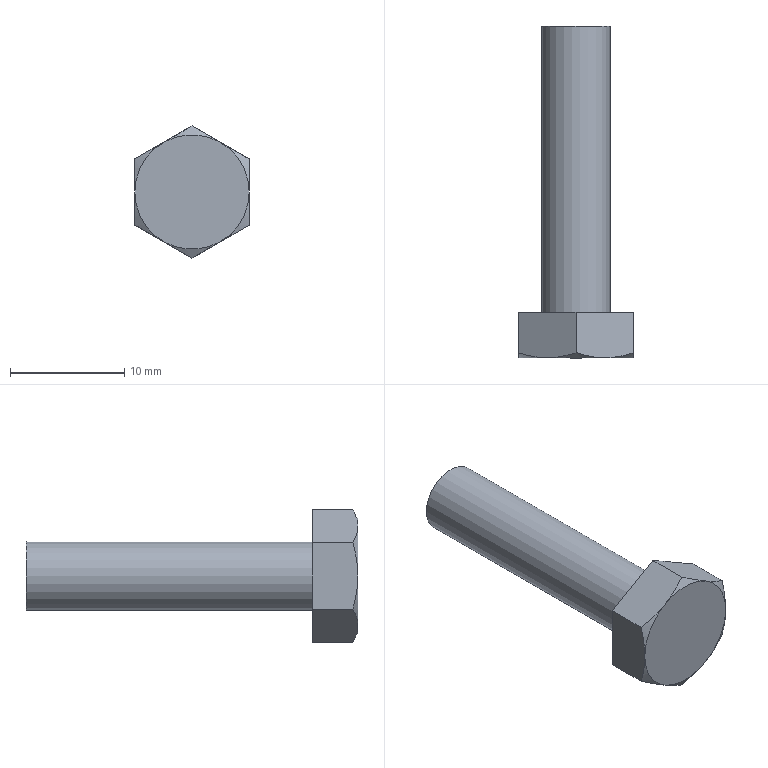Part | NX | features DATUM_CSYS 4, SKETCH 3, EXTRUDE 2, SWP104 1, SYMBOLIC_THREAD 1, UNITE 1 | 1 solid | 16 faces | box 10 x 29 x 11.547 mm | volume 1052 mm3 | plane 9 | cone 6 | cylinder 1 | commonest cylinder face diameters 6 x1
STEP:
#1=CARTESIAN_POINT('',(3.,25.,0.));
#2=VERTEX_POINT('',#1);
#3=CARTESIAN_POINT('',(0.,25.,0.));
#4=DIRECTION('',(0.,-1.,0.));
#5=DIRECTION('',(1.,0.,0.));
#6=AXIS2_PLACEMENT_3D('',#3,#4,#5);
#7=CIRCLE('',#6,3.);
#8=EDGE_CURVE('',#2,#2,#7,.T.);
#9=ORIENTED_EDGE('',*,*,#8,.T.);
#10=EDGE_LOOP('',(#9));
#11=FACE_BOUND('',#10,.T.);
#12=CARTESIAN_POINT('',(3.,0.,0.));
#13=VERTEX_POINT('',#12);
#14=CARTESIAN_POINT('',(0.,0.,0.));
#15=DIRECTION('',(0.,-1.,0.));
#16=DIRECTION('',(1.,0.,0.));
#17=AXIS2_PLACEMENT_3D('',#14,#15,#16);
#18=CIRCLE('',#17,3.);
#19=EDGE_CURVE('',#13,#13,#18,.T.);
#20=ORIENTED_EDGE('',*,*,#19,.F.);
#21=EDGE_LOOP('',(#20));
#22=FACE_BOUND('',#21,.T.);
#23=CARTESIAN_POINT('',(0.,25.,0.));
#24=DIRECTION('',(0.,-1.,0.));
#25=DIRECTION('',(0.,0.,-1.));
#26=AXIS2_PLACEMENT_3D('',#23,#24,#25);
#27=CYLINDRICAL_SURFACE('',#26,3.);
#28=ADVANCED_FACE('',(#11,#22),#27,.T.);
#29=ORIENTED_EDGE('',*,*,#8,.F.);
#30=EDGE_LOOP('',(#29));
#31=FACE_BOUND('',#30,.T.);
#32=CARTESIAN_POINT('',(0.,25.,0.));
#33=DIRECTION('',(0.,-1.,0.));
#34=DIRECTION('',(0.,0.,-1.));
#35=AXIS2_PLACEMENT_3D('',#32,#33,#34);
#36=PLANE('',#35);
#37=ADVANCED_FACE('',(#31),#36,.F.);
#38=CARTESIAN_POINT('',(-5.,-3.553,-2.887));
#39=VERTEX_POINT('',#38);
#40=CARTESIAN_POINT('',(-5.,0.,-2.887));
#41=VERTEX_POINT('',#40);
#42=CARTESIAN_POINT('',(-5.,-4.,-2.887));
#43=DIRECTION('',(0.,1.,0.));
#44=VECTOR('',#43,1000.);
#45=LINE('',#42,#44);
#46=EDGE_CURVE('',#39,#41,#45,.T.);
#47=ORIENTED_EDGE('',*,*,#46,.F.);
#48=CARTESIAN_POINT('',(-5.,-4.,0.));
#49=VERTEX_POINT('',#48);
#50=CARTESIAN_POINT('',(-5.,-3.553,-2.887));
#51=CARTESIAN_POINT('',(-5.,-3.825,-1.947));
#52=CARTESIAN_POINT('',(-5.,-4.,-0.9768));
#53=CARTESIAN_POINT('',(-5.,-4.,0.));
#54=B_SPLINE_CURVE_WITH_KNOTS('',3,(#50,#51,#52,#53),.UNSPECIFIED.,.F.,.F.,(4,4),(0.005345,0.008267),.UNSPECIFIED.);
#55=EDGE_CURVE('',#39,#49,#54,.T.);
#56=ORIENTED_EDGE('',*,*,#55,.T.);
#57=CARTESIAN_POINT('',(-5.,-3.553,2.887));
#58=VERTEX_POINT('',#57);
#59=CARTESIAN_POINT('',(-5.,-4.,0.));
#60=CARTESIAN_POINT('',(-5.,-4.,0.9775));
#61=CARTESIAN_POINT('',(-5.,-3.823,1.953));
#62=CARTESIAN_POINT('',(-5.,-3.553,2.887));
#63=B_SPLINE_CURVE_WITH_KNOTS('',3,(#59,#60,#61,#62),.UNSPECIFIED.,.F.,.F.,(4,4),(0.008267,0.01119),.UNSPECIFIED.);
#64=EDGE_CURVE('',#49,#58,#63,.T.);
#65=ORIENTED_EDGE('',*,*,#64,.T.);
#66=CARTESIAN_POINT('',(-5.,0.,2.887));
#67=VERTEX_POINT('',#66);
#68=CARTESIAN_POINT('',(-5.,-4.,2.887));
#69=DIRECTION('',(0.,1.,0.));
#70=VECTOR('',#69,1000.);
#71=LINE('',#68,#70);
#72=EDGE_CURVE('',#58,#67,#71,.T.);
#73=ORIENTED_EDGE('',*,*,#72,.T.);
#74=CARTESIAN_POINT('',(-5.,0.,2.887));
#75=DIRECTION('',(0.,0.,-1.));
#76=VECTOR('',#75,1000.);
#77=LINE('',#74,#76);
#78=EDGE_CURVE('',#67,#41,#77,.T.);
#79=ORIENTED_EDGE('',*,*,#78,.T.);
#80=EDGE_LOOP('',(#47,#56,#65,#73,#79));
#81=FACE_BOUND('',#80,.T.);
#82=CARTESIAN_POINT('',(-5.,-4.,2.887));
#83=DIRECTION('',(1.,0.,0.));
#84=DIRECTION('',(0.,0.,-1.));
#85=AXIS2_PLACEMENT_3D('',#82,#83,#84);
#86=PLANE('',#85);
#87=ADVANCED_FACE('',(#81),#86,.F.);
#88=CARTESIAN_POINT('',(0.,-3.553,-5.774));
#89=VERTEX_POINT('',#88);
#90=CARTESIAN_POINT('',(0.,0.,-5.774));
#91=VERTEX_POINT('',#90);
#92=CARTESIAN_POINT('',(0.,-4.,-5.774));
#93=DIRECTION('',(0.,1.,0.));
#94=VECTOR('',#93,1000.);
#95=LINE('',#92,#94);
#96=EDGE_CURVE('',#89,#91,#95,.T.);
#97=ORIENTED_EDGE('',*,*,#96,.F.);
#98=CARTESIAN_POINT('',(-2.5,-4.,-4.33));
#99=VERTEX_POINT('',#98);
#100=CARTESIAN_POINT('',(0.,-3.553,-5.774));
#101=CARTESIAN_POINT('',(-0.8179,-3.826,-5.301));
#102=CARTESIAN_POINT('',(-1.648,-4.,-4.822));
#103=CARTESIAN_POINT('',(-2.5,-4.,-4.33));
#104=B_SPLINE_CURVE_WITH_KNOTS('',3,(#100,#101,#102,#103),.UNSPECIFIED.,.F.,.F.,(4,4),(0.000000238,0.002921),.UNSPECIFIED.);
#105=EDGE_CURVE('',#89,#99,#104,.T.);
#106=ORIENTED_EDGE('',*,*,#105,.T.);
#107=CARTESIAN_POINT('',(-2.5,-4.,-4.33));
#108=CARTESIAN_POINT('',(-3.349,-4.,-3.84));
#109=CARTESIAN_POINT('',(-4.184,-3.825,-3.358));
#110=CARTESIAN_POINT('',(-5.,-3.553,-2.887));
#111=B_SPLINE_CURVE_WITH_KNOTS('',3,(#107,#108,#109,#110),.UNSPECIFIED.,.F.,.F.,(4,4),(0.002921,0.005831),.UNSPECIFIED.);
#112=EDGE_CURVE('',#99,#39,#111,.T.);
#113=ORIENTED_EDGE('',*,*,#112,.T.);
#114=ORIENTED_EDGE('',*,*,#46,.T.);
#115=CARTESIAN_POINT('',(-5.,0.,-2.887));
#116=DIRECTION('',(0.866,0.,-0.5));
#117=VECTOR('',#116,1000.);
#118=LINE('',#115,#117);
#119=EDGE_CURVE('',#41,#91,#118,.T.);
#120=ORIENTED_EDGE('',*,*,#119,.T.);
#121=EDGE_LOOP('',(#97,#106,#113,#114,#120));
#122=FACE_BOUND('',#121,.T.);
#123=CARTESIAN_POINT('',(-5.,-4.,-2.887));
#124=DIRECTION('',(0.5,0.,0.866));
#125=DIRECTION('',(0.866,0.,-0.5));
#126=AXIS2_PLACEMENT_3D('',#123,#124,#125);
#127=PLANE('',#126);
#128=ADVANCED_FACE('',(#122),#127,.F.);
#129=CARTESIAN_POINT('',(5.,-3.553,-2.887));
#130=VERTEX_POINT('',#129);
#131=CARTESIAN_POINT('',(5.,0.,-2.887));
#132=VERTEX_POINT('',#131);
#133=CARTESIAN_POINT('',(5.,-4.,-2.887));
#134=DIRECTION('',(0.,1.,0.));
#135=VECTOR('',#134,1000.);
#136=LINE('',#133,#135);
#137=EDGE_CURVE('',#130,#132,#136,.T.);
#138=ORIENTED_EDGE('',*,*,#137,.F.);
#139=CARTESIAN_POINT('',(2.5,-4.,-4.33));
#140=VERTEX_POINT('',#139);
#141=CARTESIAN_POINT('',(5.,-3.553,-2.887));
#142=CARTESIAN_POINT('',(4.182,-3.826,-3.359));
#143=CARTESIAN_POINT('',(3.352,-4.,-3.838));
#144=CARTESIAN_POINT('',(2.5,-4.,-4.33));
#145=B_SPLINE_CURVE_WITH_KNOTS('',3,(#141,#142,#143,#144),.UNSPECIFIED.,.F.,.F.,(4,4),(0.000000238,0.002921),.UNSPECIFIED.);
#146=EDGE_CURVE('',#130,#140,#145,.T.);
#147=ORIENTED_EDGE('',*,*,#146,.T.);
#148=CARTESIAN_POINT('',(2.5,-4.,-4.33));
#149=CARTESIAN_POINT('',(1.651,-4.,-4.82));
#150=CARTESIAN_POINT('',(0.8159,-3.825,-5.302));
#151=CARTESIAN_POINT('',(0.,-3.553,-5.774));
#152=B_SPLINE_CURVE_WITH_KNOTS('',3,(#148,#149,#150,#151),.UNSPECIFIED.,.F.,.F.,(4,4),(0.002921,0.005831),.UNSPECIFIED.);
#153=EDGE_CURVE('',#140,#89,#152,.T.);
#154=ORIENTED_EDGE('',*,*,#153,.T.);
#155=ORIENTED_EDGE('',*,*,#96,.T.);
#156=CARTESIAN_POINT('',(0.,0.,-5.774));
#157=DIRECTION('',(0.866,0.,0.5));
#158=VECTOR('',#157,1000.);
#159=LINE('',#156,#158);
#160=EDGE_CURVE('',#91,#132,#159,.T.);
#161=ORIENTED_EDGE('',*,*,#160,.T.);
#162=EDGE_LOOP('',(#138,#147,#154,#155,#161));
#163=FACE_BOUND('',#162,.T.);
#164=CARTESIAN_POINT('',(0.,-4.,-5.774));
#165=DIRECTION('',(-0.5,0.,0.866));
#166=DIRECTION('',(0.866,0.,0.5));
#167=AXIS2_PLACEMENT_3D('',#164,#165,#166);
#168=PLANE('',#167);
#169=ADVANCED_FACE('',(#163),#168,.F.);
#170=CARTESIAN_POINT('',(5.,-3.553,2.887));
#171=VERTEX_POINT('',#170);
#172=CARTESIAN_POINT('',(5.,0.,2.887));
#173=VERTEX_POINT('',#172);
#174=CARTESIAN_POINT('',(5.,-4.,2.887));
#175=DIRECTION('',(0.,1.,0.));
#176=VECTOR('',#175,1000.);
#177=LINE('',#174,#176);
#178=EDGE_CURVE('',#171,#173,#177,.T.);
#179=ORIENTED_EDGE('',*,*,#178,.F.);
#180=CARTESIAN_POINT('',(5.,-4.,0.));
#181=VERTEX_POINT('',#180);
#182=CARTESIAN_POINT('',(5.,-4.,0.));
#183=CARTESIAN_POINT('',(5.,-4.,0.9775));
#184=CARTESIAN_POINT('',(5.,-3.823,1.953));
#185=CARTESIAN_POINT('',(5.,-3.553,2.887));
#186=B_SPLINE_CURVE_WITH_KNOTS('',3,(#182,#183,#184,#185),.UNSPECIFIED.,.F.,.F.,(4,4),(0.008267,0.01119),.UNSPECIFIED.);
#187=EDGE_CURVE('',#171,#181,#186,.F.);
#188=ORIENTED_EDGE('',*,*,#187,.T.);
#189=CARTESIAN_POINT('',(5.,-3.553,-2.887));
#190=CARTESIAN_POINT('',(5.,-3.825,-1.947));
#191=CARTESIAN_POINT('',(5.,-4.,-0.9768));
#192=CARTESIAN_POINT('',(5.,-4.,0.));
#193=B_SPLINE_CURVE_WITH_KNOTS('',3,(#189,#190,#191,#192),.UNSPECIFIED.,.F.,.F.,(4,4),(0.005345,0.008267),.UNSPECIFIED.);
#194=EDGE_CURVE('',#181,#130,#193,.F.);
#195=ORIENTED_EDGE('',*,*,#194,.T.);
#196=ORIENTED_EDGE('',*,*,#137,.T.);
#197=CARTESIAN_POINT('',(5.,0.,-2.887));
#198=DIRECTION('',(0.,0.,1.));
#199=VECTOR('',#198,1000.);
#200=LINE('',#197,#199);
#201=EDGE_CURVE('',#132,#173,#200,.T.);
#202=ORIENTED_EDGE('',*,*,#201,.T.);
#203=EDGE_LOOP('',(#179,#188,#195,#196,#202));
#204=FACE_BOUND('',#203,.T.);
#205=CARTESIAN_POINT('',(5.,-4.,-2.887));
#206=DIRECTION('',(-1.,0.,0.));
#207=DIRECTION('',(0.,0.,1.));
#208=AXIS2_PLACEMENT_3D('',#205,#206,#207);
#209=PLANE('',#208);
#210=ADVANCED_FACE('',(#204),#209,.F.);
#211=CARTESIAN_POINT('',(0.,-3.553,5.774));
#212=VERTEX_POINT('',#211);
#213=CARTESIAN_POINT('',(0.,0.,5.774));
#214=VERTEX_POINT('',#213);
#215=CARTESIAN_POINT('',(0.,-4.,5.774));
#216=DIRECTION('',(0.,1.,0.));
#217=VECTOR('',#216,1000.);
#218=LINE('',#215,#217);
#219=EDGE_CURVE('',#212,#214,#218,.T.);
#220=ORIENTED_EDGE('',*,*,#219,.F.);
#221=CARTESIAN_POINT('',(2.5,-4.,4.33));
#222=VERTEX_POINT('',#221);
#223=CARTESIAN_POINT('',(0.,-3.553,5.774));
#224=CARTESIAN_POINT('',(0.8179,-3.826,5.301));
#225=CARTESIAN_POINT('',(1.648,-4.,4.822));
#226=CARTESIAN_POINT('',(2.5,-4.,4.33));
#227=B_SPLINE_CURVE_WITH_KNOTS('',3,(#223,#224,#225,#226),.UNSPECIFIED.,.F.,.F.,(4,4),(0.000000238,0.002921),.UNSPECIFIED.);
#228=EDGE_CURVE('',#212,#222,#227,.T.);
#229=ORIENTED_EDGE('',*,*,#228,.T.);
#230=CARTESIAN_POINT('',(2.5,-4.,4.33));
#231=CARTESIAN_POINT('',(3.349,-4.,3.84));
#232=CARTESIAN_POINT('',(4.184,-3.825,3.358));
#233=CARTESIAN_POINT('',(5.,-3.553,2.887));
#234=B_SPLINE_CURVE_WITH_KNOTS('',3,(#230,#231,#232,#233),.UNSPECIFIED.,.F.,.F.,(4,4),(0.002921,0.005831),.UNSPECIFIED.);
#235=EDGE_CURVE('',#222,#171,#234,.T.);
#236=ORIENTED_EDGE('',*,*,#235,.T.);
#237=ORIENTED_EDGE('',*,*,#178,.T.);
#238=CARTESIAN_POINT('',(5.,0.,2.887));
#239=DIRECTION('',(-0.866,0.,0.5));
#240=VECTOR('',#239,1000.);
#241=LINE('',#238,#240);
#242=EDGE_CURVE('',#173,#214,#241,.T.);
#243=ORIENTED_EDGE('',*,*,#242,.T.);
#244=EDGE_LOOP('',(#220,#229,#236,#237,#243));
#245=FACE_BOUND('',#244,.T.);
#246=CARTESIAN_POINT('',(5.,-4.,2.887));
#247=DIRECTION('',(-0.5,0.,-0.866));
#248=DIRECTION('',(-0.866,0.,0.5));
#249=AXIS2_PLACEMENT_3D('',#246,#247,#248);
#250=PLANE('',#249);
#251=ADVANCED_FACE('',(#245),#250,.F.);
#252=ORIENTED_EDGE('',*,*,#72,.F.);
#253=CARTESIAN_POINT('',(-2.5,-4.,4.33));
#254=VERTEX_POINT('',#253);
#255=CARTESIAN_POINT('',(-5.,-3.553,2.887));
#256=CARTESIAN_POINT('',(-4.182,-3.826,3.359));
#257=CARTESIAN_POINT('',(-3.352,-4.,3.838));
#258=CARTESIAN_POINT('',(-2.5,-4.,4.33));
#259=B_SPLINE_CURVE_WITH_KNOTS('',3,(#255,#256,#257,#258),.UNSPECIFIED.,.F.,.F.,(4,4),(0.000000238,0.002921),.UNSPECIFIED.);
#260=EDGE_CURVE('',#58,#254,#259,.T.);
#261=ORIENTED_EDGE('',*,*,#260,.T.);
#262=CARTESIAN_POINT('',(-2.5,-4.,4.33));
#263=CARTESIAN_POINT('',(-1.651,-4.,4.82));
#264=CARTESIAN_POINT('',(-0.8159,-3.825,5.302));
#265=CARTESIAN_POINT('',(0.,-3.553,5.774));
#266=B_SPLINE_CURVE_WITH_KNOTS('',3,(#262,#263,#264,#265),.UNSPECIFIED.,.F.,.F.,(4,4),(0.002921,0.005831),.UNSPECIFIED.);
#267=EDGE_CURVE('',#254,#212,#266,.T.);
#268=ORIENTED_EDGE('',*,*,#267,.T.);
#269=ORIENTED_EDGE('',*,*,#219,.T.);
#270=CARTESIAN_POINT('',(0.,0.,5.774));
#271=DIRECTION('',(-0.866,0.,-0.5));
#272=VECTOR('',#271,1000.);
#273=LINE('',#270,#272);
#274=EDGE_CURVE('',#214,#67,#273,.T.);
#275=ORIENTED_EDGE('',*,*,#274,.T.);
#276=EDGE_LOOP('',(#252,#261,#268,#269,#275));
#277=FACE_BOUND('',#276,.T.);
#278=CARTESIAN_POINT('',(0.,-4.,5.774));
#279=DIRECTION('',(0.5,0.,-0.866));
#280=DIRECTION('',(-0.866,0.,-0.5));
#281=AXIS2_PLACEMENT_3D('',#278,#279,#280);
#282=PLANE('',#281);
#283=ADVANCED_FACE('',(#277),#282,.F.);
#284=ORIENTED_EDGE('',*,*,#19,.T.);
#285=EDGE_LOOP('',(#284));
#286=FACE_BOUND('',#285,.T.);
#287=ORIENTED_EDGE('',*,*,#78,.F.);
#288=ORIENTED_EDGE('',*,*,#274,.F.);
#289=ORIENTED_EDGE('',*,*,#242,.F.);
#290=ORIENTED_EDGE('',*,*,#201,.F.);
#291=ORIENTED_EDGE('',*,*,#160,.F.);
#292=ORIENTED_EDGE('',*,*,#119,.F.);
#293=EDGE_LOOP('',(#287,#288,#289,#290,#291,#292));
#294=FACE_BOUND('',#293,.T.);
#295=CARTESIAN_POINT('',(0.,0.,0.));
#296=DIRECTION('',(0.,-1.,0.));
#297=DIRECTION('',(0.,0.,-1.));
#298=AXIS2_PLACEMENT_3D('',#295,#296,#297);
#299=PLANE('',#298);
#300=ADVANCED_FACE('',(#286,#294),#299,.F.);
#301=ORIENTED_EDGE('',*,*,#267,.F.);
#302=CARTESIAN_POINT('',(0.,-4.,0.));
#303=DIRECTION('',(0.,-1.,0.));
#304=DIRECTION('',(0.,0.,-1.));
#305=AXIS2_PLACEMENT_3D('',#302,#303,#304);
#306=CIRCLE('',#305,5.);
#307=EDGE_CURVE('',#222,#254,#306,.T.);
#308=ORIENTED_EDGE('',*,*,#307,.F.);
#309=ORIENTED_EDGE('',*,*,#228,.F.);
#310=EDGE_LOOP('',(#301,#308,#309));
#311=FACE_BOUND('',#310,.T.);
#312=CARTESIAN_POINT('',(0.,-2.3,0.));
#313=DIRECTION('',(0.,1.,0.));
#314=DIRECTION('',(0.,0.,1.));
#315=AXIS2_PLACEMENT_3D('',#312,#313,#314);
#316=CONICAL_SURFACE('',#315,7.944,1.047);
#317=ADVANCED_FACE('',(#311),#316,.T.);
#318=CARTESIAN_POINT('',(0.,-4.,0.));
#319=DIRECTION('',(0.,-1.,0.));
#320=DIRECTION('',(0.,0.,-1.));
#321=AXIS2_PLACEMENT_3D('',#318,#319,#320);
#322=CIRCLE('',#321,5.);
#323=EDGE_CURVE('',#254,#49,#322,.T.);
#324=ORIENTED_EDGE('',*,*,#323,.F.);
#325=ORIENTED_EDGE('',*,*,#260,.F.);
#326=ORIENTED_EDGE('',*,*,#64,.F.);
#327=EDGE_LOOP('',(#324,#325,#326));
#328=FACE_BOUND('',#327,.T.);
#329=CARTESIAN_POINT('',(0.,-2.3,0.));
#330=DIRECTION('',(0.,1.,0.));
#331=DIRECTION('',(0.,0.,1.));
#332=AXIS2_PLACEMENT_3D('',#329,#330,#331);
#333=CONICAL_SURFACE('',#332,7.944,1.047);
#334=ADVANCED_FACE('',(#328),#333,.T.);
#335=ORIENTED_EDGE('',*,*,#235,.F.);
#336=CARTESIAN_POINT('',(0.,-4.,0.));
#337=DIRECTION('',(0.,-1.,0.));
#338=DIRECTION('',(0.,0.,-1.));
#339=AXIS2_PLACEMENT_3D('',#336,#337,#338);
#340=CIRCLE('',#339,5.);
#341=EDGE_CURVE('',#181,#222,#340,.T.);
#342=ORIENTED_EDGE('',*,*,#341,.F.);
#343=ORIENTED_EDGE('',*,*,#187,.F.);
#344=EDGE_LOOP('',(#335,#342,#343));
#345=FACE_BOUND('',#344,.T.);
#346=CARTESIAN_POINT('',(0.,-2.3,0.));
#347=DIRECTION('',(0.,1.,0.));
#348=DIRECTION('',(0.,0.,1.));
#349=AXIS2_PLACEMENT_3D('',#346,#347,#348);
#350=CONICAL_SURFACE('',#349,7.944,1.047);
#351=ADVANCED_FACE('',(#345),#350,.T.);
#352=ORIENTED_EDGE('',*,*,#194,.F.);
#353=CARTESIAN_POINT('',(0.,-4.,0.));
#354=DIRECTION('',(0.,-1.,0.));
#355=DIRECTION('',(0.,0.,-1.));
#356=AXIS2_PLACEMENT_3D('',#353,#354,#355);
#357=CIRCLE('',#356,5.);
#358=EDGE_CURVE('',#140,#181,#357,.T.);
#359=ORIENTED_EDGE('',*,*,#358,.F.);
#360=ORIENTED_EDGE('',*,*,#146,.F.);
#361=EDGE_LOOP('',(#352,#359,#360));
#362=FACE_BOUND('',#361,.T.);
#363=CARTESIAN_POINT('',(0.,-2.3,0.));
#364=DIRECTION('',(0.,1.,0.));
#365=DIRECTION('',(0.,0.,1.));
#366=AXIS2_PLACEMENT_3D('',#363,#364,#365);
#367=CONICAL_SURFACE('',#366,7.944,1.047);
#368=ADVANCED_FACE('',(#362),#367,.T.);
#369=CARTESIAN_POINT('',(0.,-4.,0.));
#370=DIRECTION('',(0.,-1.,0.));
#371=DIRECTION('',(0.,0.,-1.));
#372=AXIS2_PLACEMENT_3D('',#369,#370,#371);
#373=CIRCLE('',#372,5.);
#374=EDGE_CURVE('',#99,#140,#373,.T.);
#375=ORIENTED_EDGE('',*,*,#374,.F.);
#376=ORIENTED_EDGE('',*,*,#105,.F.);
#377=ORIENTED_EDGE('',*,*,#153,.F.);
#378=EDGE_LOOP('',(#375,#376,#377));
#379=FACE_BOUND('',#378,.T.);
#380=CARTESIAN_POINT('',(0.,-2.3,0.));
#381=DIRECTION('',(0.,1.,0.));
#382=DIRECTION('',(0.,0.,1.));
#383=AXIS2_PLACEMENT_3D('',#380,#381,#382);
#384=CONICAL_SURFACE('',#383,7.944,1.047);
#385=ADVANCED_FACE('',(#379),#384,.T.);
#386=CARTESIAN_POINT('',(0.,-4.,0.));
#387=DIRECTION('',(0.,-1.,0.));
#388=DIRECTION('',(0.,0.,-1.));
#389=AXIS2_PLACEMENT_3D('',#386,#387,#388);
#390=CIRCLE('',#389,5.);
#391=EDGE_CURVE('',#49,#99,#390,.T.);
#392=ORIENTED_EDGE('',*,*,#391,.F.);
#393=ORIENTED_EDGE('',*,*,#55,.F.);
#394=ORIENTED_EDGE('',*,*,#112,.F.);
#395=EDGE_LOOP('',(#392,#393,#394));
#396=FACE_BOUND('',#395,.T.);
#397=CARTESIAN_POINT('',(0.,-2.3,0.));
#398=DIRECTION('',(0.,1.,0.));
#399=DIRECTION('',(0.,0.,1.));
#400=AXIS2_PLACEMENT_3D('',#397,#398,#399);
#401=CONICAL_SURFACE('',#400,7.944,1.047);
#402=ADVANCED_FACE('',(#396),#401,.T.);
#403=ORIENTED_EDGE('',*,*,#374,.T.);
#404=ORIENTED_EDGE('',*,*,#358,.T.);
#405=ORIENTED_EDGE('',*,*,#341,.T.);
#406=ORIENTED_EDGE('',*,*,#307,.T.);
#407=ORIENTED_EDGE('',*,*,#323,.T.);
#408=ORIENTED_EDGE('',*,*,#391,.T.);
#409=EDGE_LOOP('',(#403,#404,#405,#406,#407,#408));
#410=FACE_BOUND('',#409,.T.);
#411=CARTESIAN_POINT('',(0.,-4.,0.));
#412=DIRECTION('',(0.,-1.,0.));
#413=DIRECTION('',(0.,0.,-1.));
#414=AXIS2_PLACEMENT_3D('',#411,#412,#413);
#415=PLANE('',#414);
#416=ADVANCED_FACE('',(#410),#415,.T.);
#417=CLOSED_SHELL('',(#28,#37,#87,#128,#169,#210,#251,#283,#300,#317,#334,#351,#368,#385,#402,#416));
#418=MANIFOLD_SOLID_BREP('',#417);
#419=(LENGTH_UNIT()NAMED_UNIT(*)SI_UNIT(.MILLI.,.METRE.));
#420=UNCERTAINTY_MEASURE_WITH_UNIT(LENGTH_MEASURE(0.0508),#419,'','');
#421=(NAMED_UNIT(*)PLANE_ANGLE_UNIT()SI_UNIT($,.RADIAN.));
#422=(NAMED_UNIT(*)SI_UNIT($,.STERADIAN.)SOLID_ANGLE_UNIT());
#423=(GEOMETRIC_REPRESENTATION_CONTEXT(3)GLOBAL_UNCERTAINTY_ASSIGNED_CONTEXT((#420))GLOBAL_UNIT_ASSIGNED_CONTEXT((#419,#421,#422))REPRESENTATION_CONTEXT('',''));
#424=ADVANCED_BREP_SHAPE_REPRESENTATION('',(#418),#423);